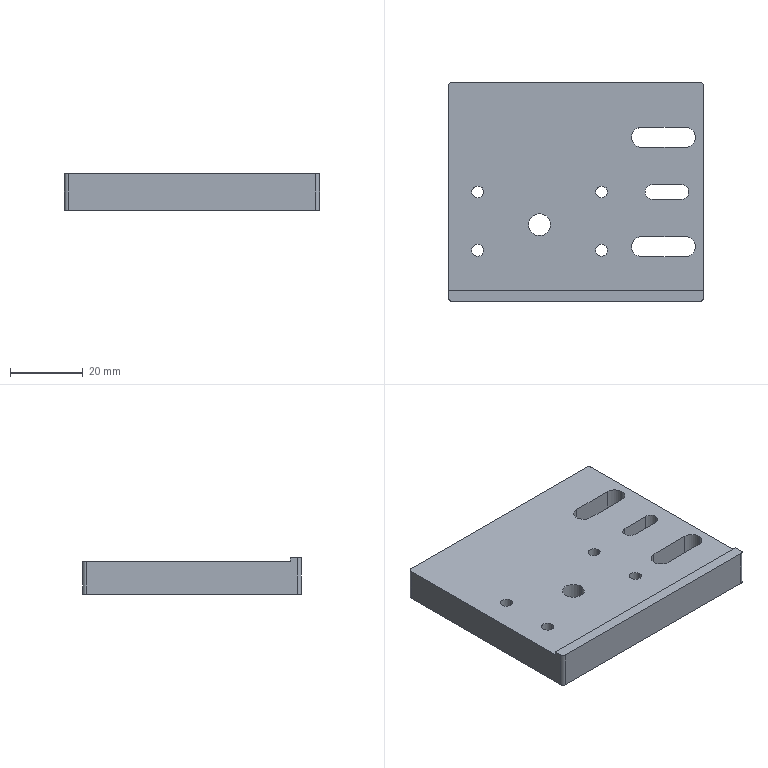Part | STEP file | 04-13 support plate A | 1 solid | 37 faces | box 70 x 60 x 10 mm | volume 35423 mm3 | cylinder 23 | plane 14 | commonest cylinder face diameters 3.3 x8 5.5 x6 2 x4 4 x3 6 x2
STEP:
#1=CARTESIAN_POINT('',(31.,0.,0.));
#2=VERTEX_POINT('',#1);
#3=CARTESIAN_POINT('',(29.,2.,0.));
#4=VERTEX_POINT('',#3);
#5=CARTESIAN_POINT('',(29.,0.,0.));
#6=DIRECTION('',(0.,0.,1.));
#7=DIRECTION('',(1.,0.,0.));
#8=AXIS2_PLACEMENT_3D('',#5,#6,#7);
#9=CIRCLE('',#8,2.);
#10=EDGE_CURVE('',#2,#4,#9,.T.);
#11=ORIENTED_EDGE('',*,*,#10,.F.);
#12=CARTESIAN_POINT('',(31.,0.,9.));
#13=VERTEX_POINT('',#12);
#14=CARTESIAN_POINT('',(31.,0.,-65.));
#15=DIRECTION('',(0.,0.,1.));
#16=VECTOR('',#15,1000.);
#17=LINE('',#14,#16);
#18=EDGE_CURVE('',#2,#13,#17,.T.);
#19=ORIENTED_EDGE('',*,*,#18,.T.);
#20=CARTESIAN_POINT('',(29.,2.,9.));
#21=VERTEX_POINT('',#20);
#22=CARTESIAN_POINT('',(29.,0.,9.));
#23=DIRECTION('',(0.,0.,1.));
#24=DIRECTION('',(1.,0.,0.));
#25=AXIS2_PLACEMENT_3D('',#22,#23,#24);
#26=CIRCLE('',#25,2.);
#27=EDGE_CURVE('',#13,#21,#26,.T.);
#28=ORIENTED_EDGE('',*,*,#27,.T.);
#29=CARTESIAN_POINT('',(29.,2.,-65.));
#30=DIRECTION('',(0.,0.,1.));
#31=VECTOR('',#30,1000.);
#32=LINE('',#29,#31);
#33=EDGE_CURVE('',#4,#21,#32,.T.);
#34=ORIENTED_EDGE('',*,*,#33,.F.);
#35=EDGE_LOOP('',(#11,#19,#28,#34));
#36=FACE_OUTER_BOUND('',#35,.T.);
#37=CARTESIAN_POINT('',(29.,0.,-65.));
#38=DIRECTION('',(0.,0.,1.));
#39=DIRECTION('',(1.,0.,0.));
#40=AXIS2_PLACEMENT_3D('',#37,#38,#39);
#41=CYLINDRICAL_SURFACE('',#40,2.);
#42=ADVANCED_FACE('',(#36),#41,.F.);
#43=CARTESIAN_POINT('',(32.75,15.,0.));
#44=VERTEX_POINT('',#43);
#45=CARTESIAN_POINT('',(30.,17.75,0.));
#46=VERTEX_POINT('',#45);
#47=CARTESIAN_POINT('',(30.,15.,0.));
#48=DIRECTION('',(0.,0.,1.));
#49=DIRECTION('',(1.,0.,0.));
#50=AXIS2_PLACEMENT_3D('',#47,#48,#49);
#51=CIRCLE('',#50,2.75);
#52=EDGE_CURVE('',#44,#46,#51,.T.);
#53=ORIENTED_EDGE('',*,*,#52,.F.);
#54=CARTESIAN_POINT('',(32.75,15.,9.));
#55=VERTEX_POINT('',#54);
#56=CARTESIAN_POINT('',(32.75,15.,-65.));
#57=DIRECTION('',(0.,0.,1.));
#58=VECTOR('',#57,1000.);
#59=LINE('',#56,#58);
#60=EDGE_CURVE('',#44,#55,#59,.T.);
#61=ORIENTED_EDGE('',*,*,#60,.T.);
#62=CARTESIAN_POINT('',(30.,17.75,9.));
#63=VERTEX_POINT('',#62);
#64=CARTESIAN_POINT('',(30.,15.,9.));
#65=DIRECTION('',(0.,0.,1.));
#66=DIRECTION('',(-1.,0.,0.));
#67=AXIS2_PLACEMENT_3D('',#64,#65,#66);
#68=CIRCLE('',#67,2.75);
#69=EDGE_CURVE('',#55,#63,#68,.T.);
#70=ORIENTED_EDGE('',*,*,#69,.T.);
#71=CARTESIAN_POINT('',(30.,17.75,-65.));
#72=DIRECTION('',(0.,0.,1.));
#73=VECTOR('',#72,1000.);
#74=LINE('',#71,#73);
#75=EDGE_CURVE('',#46,#63,#74,.T.);
#76=ORIENTED_EDGE('',*,*,#75,.F.);
#77=EDGE_LOOP('',(#53,#61,#70,#76));
#78=FACE_OUTER_BOUND('',#77,.T.);
#79=CARTESIAN_POINT('',(30.,15.,-65.));
#80=DIRECTION('',(0.,0.,1.));
#81=DIRECTION('',(1.,0.,0.));
#82=AXIS2_PLACEMENT_3D('',#79,#80,#81);
#83=CYLINDRICAL_SURFACE('',#82,2.75);
#84=ADVANCED_FACE('',(#78),#83,.F.);
#85=CARTESIAN_POINT('',(32.75,-15.,0.));
#86=VERTEX_POINT('',#85);
#87=CARTESIAN_POINT('',(30.,-12.25,0.));
#88=VERTEX_POINT('',#87);
#89=CARTESIAN_POINT('',(30.,-15.,0.));
#90=DIRECTION('',(0.,0.,1.));
#91=DIRECTION('',(1.,0.,0.));
#92=AXIS2_PLACEMENT_3D('',#89,#90,#91);
#93=CIRCLE('',#92,2.75);
#94=EDGE_CURVE('',#86,#88,#93,.T.);
#95=ORIENTED_EDGE('',*,*,#94,.F.);
#96=CARTESIAN_POINT('',(32.75,-15.,9.));
#97=VERTEX_POINT('',#96);
#98=CARTESIAN_POINT('',(32.75,-15.,-65.));
#99=DIRECTION('',(0.,0.,1.));
#100=VECTOR('',#99,1000.);
#101=LINE('',#98,#100);
#102=EDGE_CURVE('',#86,#97,#101,.T.);
#103=ORIENTED_EDGE('',*,*,#102,.T.);
#104=CARTESIAN_POINT('',(30.,-12.25,9.));
#105=VERTEX_POINT('',#104);
#106=CARTESIAN_POINT('',(30.,-15.,9.));
#107=DIRECTION('',(0.,0.,1.));
#108=DIRECTION('',(1.,0.,0.));
#109=AXIS2_PLACEMENT_3D('',#106,#107,#108);
#110=CIRCLE('',#109,2.75);
#111=EDGE_CURVE('',#97,#105,#110,.T.);
#112=ORIENTED_EDGE('',*,*,#111,.T.);
#113=CARTESIAN_POINT('',(30.,-12.25,-65.));
#114=DIRECTION('',(0.,0.,1.));
#115=VECTOR('',#114,1000.);
#116=LINE('',#113,#115);
#117=EDGE_CURVE('',#88,#105,#116,.T.);
#118=ORIENTED_EDGE('',*,*,#117,.F.);
#119=EDGE_LOOP('',(#95,#103,#112,#118));
#120=FACE_OUTER_BOUND('',#119,.T.);
#121=CARTESIAN_POINT('',(30.,-15.,-65.));
#122=DIRECTION('',(0.,0.,1.));
#123=DIRECTION('',(1.,0.,0.));
#124=AXIS2_PLACEMENT_3D('',#121,#122,#123);
#125=CYLINDRICAL_SURFACE('',#124,2.75);
#126=ADVANCED_FACE('',(#120),#125,.F.);
#127=CARTESIAN_POINT('',(-28.65,0.,0.));
#128=VERTEX_POINT('',#127);
#129=CARTESIAN_POINT('',(-25.35,0.,0.));
#130=VERTEX_POINT('',#129);
#131=CARTESIAN_POINT('',(-27.,0.,0.));
#132=DIRECTION('',(0.,0.,1.));
#133=DIRECTION('',(1.,0.,0.));
#134=AXIS2_PLACEMENT_3D('',#131,#132,#133);
#135=CIRCLE('',#134,1.65);
#136=EDGE_CURVE('',#128,#130,#135,.T.);
#137=ORIENTED_EDGE('',*,*,#136,.F.);
#138=CARTESIAN_POINT('',(-28.65,0.,9.));
#139=VERTEX_POINT('',#138);
#140=CARTESIAN_POINT('',(-28.65,0.,9.));
#141=DIRECTION('',(0.,0.,1.));
#142=VECTOR('',#141,1000.);
#143=LINE('',#140,#142);
#144=EDGE_CURVE('',#128,#139,#143,.T.);
#145=ORIENTED_EDGE('',*,*,#144,.T.);
#146=CARTESIAN_POINT('',(-25.35,0.,9.));
#147=VERTEX_POINT('',#146);
#148=CARTESIAN_POINT('',(-27.,0.,9.));
#149=DIRECTION('',(0.,0.,1.));
#150=DIRECTION('',(1.,0.,0.));
#151=AXIS2_PLACEMENT_3D('',#148,#149,#150);
#152=CIRCLE('',#151,1.65);
#153=EDGE_CURVE('',#139,#147,#152,.T.);
#154=ORIENTED_EDGE('',*,*,#153,.T.);
#155=CARTESIAN_POINT('',(-25.35,0.,9.));
#156=DIRECTION('',(0.,0.,1.));
#157=VECTOR('',#156,1000.);
#158=LINE('',#155,#157);
#159=EDGE_CURVE('',#130,#147,#158,.T.);
#160=ORIENTED_EDGE('',*,*,#159,.F.);
#161=EDGE_LOOP('',(#137,#145,#154,#160));
#162=FACE_OUTER_BOUND('',#161,.T.);
#163=CARTESIAN_POINT('',(-27.,0.,9.));
#164=DIRECTION('',(0.,0.,1.));
#165=DIRECTION('',(1.,0.,0.));
#166=AXIS2_PLACEMENT_3D('',#163,#164,#165);
#167=CYLINDRICAL_SURFACE('',#166,1.65);
#168=ADVANCED_FACE('',(#162),#167,.F.);
#169=CARTESIAN_POINT('',(-28.65,-16.,0.));
#170=VERTEX_POINT('',#169);
#171=CARTESIAN_POINT('',(-25.35,-16.,0.));
#172=VERTEX_POINT('',#171);
#173=CARTESIAN_POINT('',(-27.,-16.,0.));
#174=DIRECTION('',(0.,0.,1.));
#175=DIRECTION('',(1.,0.,0.));
#176=AXIS2_PLACEMENT_3D('',#173,#174,#175);
#177=CIRCLE('',#176,1.65);
#178=EDGE_CURVE('',#170,#172,#177,.T.);
#179=ORIENTED_EDGE('',*,*,#178,.F.);
#180=CARTESIAN_POINT('',(-28.65,-16.,9.));
#181=VERTEX_POINT('',#180);
#182=CARTESIAN_POINT('',(-28.65,-16.,9.));
#183=DIRECTION('',(0.,0.,1.));
#184=VECTOR('',#183,1000.);
#185=LINE('',#182,#184);
#186=EDGE_CURVE('',#170,#181,#185,.T.);
#187=ORIENTED_EDGE('',*,*,#186,.T.);
#188=CARTESIAN_POINT('',(-25.35,-16.,9.));
#189=VERTEX_POINT('',#188);
#190=CARTESIAN_POINT('',(-27.,-16.,9.));
#191=DIRECTION('',(0.,0.,1.));
#192=DIRECTION('',(1.,0.,0.));
#193=AXIS2_PLACEMENT_3D('',#190,#191,#192);
#194=CIRCLE('',#193,1.65);
#195=EDGE_CURVE('',#181,#189,#194,.T.);
#196=ORIENTED_EDGE('',*,*,#195,.T.);
#197=CARTESIAN_POINT('',(-25.35,-16.,9.));
#198=DIRECTION('',(0.,0.,1.));
#199=VECTOR('',#198,1000.);
#200=LINE('',#197,#199);
#201=EDGE_CURVE('',#172,#189,#200,.T.);
#202=ORIENTED_EDGE('',*,*,#201,.F.);
#203=EDGE_LOOP('',(#179,#187,#196,#202));
#204=FACE_OUTER_BOUND('',#203,.T.);
#205=CARTESIAN_POINT('',(-27.,-16.,9.));
#206=DIRECTION('',(0.,0.,1.));
#207=DIRECTION('',(1.,0.,0.));
#208=AXIS2_PLACEMENT_3D('',#205,#206,#207);
#209=CYLINDRICAL_SURFACE('',#208,1.65);
#210=ADVANCED_FACE('',(#204),#209,.F.);
#211=CARTESIAN_POINT('',(5.35,0.,0.));
#212=VERTEX_POINT('',#211);
#213=CARTESIAN_POINT('',(8.65,0.,0.));
#214=VERTEX_POINT('',#213);
#215=CARTESIAN_POINT('',(7.,0.,0.));
#216=DIRECTION('',(0.,0.,1.));
#217=DIRECTION('',(1.,0.,0.));
#218=AXIS2_PLACEMENT_3D('',#215,#216,#217);
#219=CIRCLE('',#218,1.65);
#220=EDGE_CURVE('',#212,#214,#219,.T.);
#221=ORIENTED_EDGE('',*,*,#220,.F.);
#222=CARTESIAN_POINT('',(5.35,0.,9.));
#223=VERTEX_POINT('',#222);
#224=CARTESIAN_POINT('',(5.35,0.,9.));
#225=DIRECTION('',(0.,0.,1.));
#226=VECTOR('',#225,1000.);
#227=LINE('',#224,#226);
#228=EDGE_CURVE('',#212,#223,#227,.T.);
#229=ORIENTED_EDGE('',*,*,#228,.T.);
#230=CARTESIAN_POINT('',(8.65,0.,9.));
#231=VERTEX_POINT('',#230);
#232=CARTESIAN_POINT('',(7.,0.,9.));
#233=DIRECTION('',(0.,0.,1.));
#234=DIRECTION('',(1.,0.,0.));
#235=AXIS2_PLACEMENT_3D('',#232,#233,#234);
#236=CIRCLE('',#235,1.65);
#237=EDGE_CURVE('',#223,#231,#236,.T.);
#238=ORIENTED_EDGE('',*,*,#237,.T.);
#239=CARTESIAN_POINT('',(8.65,0.,9.));
#240=DIRECTION('',(0.,0.,1.));
#241=VECTOR('',#240,1000.);
#242=LINE('',#239,#241);
#243=EDGE_CURVE('',#214,#231,#242,.T.);
#244=ORIENTED_EDGE('',*,*,#243,.F.);
#245=EDGE_LOOP('',(#221,#229,#238,#244));
#246=FACE_OUTER_BOUND('',#245,.T.);
#247=CARTESIAN_POINT('',(7.,0.,9.));
#248=DIRECTION('',(0.,0.,1.));
#249=DIRECTION('',(1.,0.,0.));
#250=AXIS2_PLACEMENT_3D('',#247,#248,#249);
#251=CYLINDRICAL_SURFACE('',#250,1.65);
#252=ADVANCED_FACE('',(#246),#251,.F.);
#253=CARTESIAN_POINT('',(5.35,-16.,0.));
#254=VERTEX_POINT('',#253);
#255=CARTESIAN_POINT('',(8.65,-16.,0.));
#256=VERTEX_POINT('',#255);
#257=CARTESIAN_POINT('',(7.,-16.,0.));
#258=DIRECTION('',(0.,0.,1.));
#259=DIRECTION('',(1.,0.,0.));
#260=AXIS2_PLACEMENT_3D('',#257,#258,#259);
#261=CIRCLE('',#260,1.65);
#262=EDGE_CURVE('',#254,#256,#261,.T.);
#263=ORIENTED_EDGE('',*,*,#262,.F.);
#264=CARTESIAN_POINT('',(5.35,-16.,9.));
#265=VERTEX_POINT('',#264);
#266=CARTESIAN_POINT('',(5.35,-16.,9.));
#267=DIRECTION('',(0.,0.,1.));
#268=VECTOR('',#267,1000.);
#269=LINE('',#266,#268);
#270=EDGE_CURVE('',#254,#265,#269,.T.);
#271=ORIENTED_EDGE('',*,*,#270,.T.);
#272=CARTESIAN_POINT('',(8.65,-16.,9.));
#273=VERTEX_POINT('',#272);
#274=CARTESIAN_POINT('',(7.,-16.,9.));
#275=DIRECTION('',(0.,0.,1.));
#276=DIRECTION('',(1.,0.,0.));
#277=AXIS2_PLACEMENT_3D('',#274,#275,#276);
#278=CIRCLE('',#277,1.65);
#279=EDGE_CURVE('',#265,#273,#278,.T.);
#280=ORIENTED_EDGE('',*,*,#279,.T.);
#281=CARTESIAN_POINT('',(8.65,-16.,9.));
#282=DIRECTION('',(0.,0.,1.));
#283=VECTOR('',#282,1000.);
#284=LINE('',#281,#283);
#285=EDGE_CURVE('',#256,#273,#284,.T.);
#286=ORIENTED_EDGE('',*,*,#285,.F.);
#287=EDGE_LOOP('',(#263,#271,#280,#286));
#288=FACE_OUTER_BOUND('',#287,.T.);
#289=CARTESIAN_POINT('',(7.,-16.,9.));
#290=DIRECTION('',(0.,0.,1.));
#291=DIRECTION('',(1.,0.,0.));
#292=AXIS2_PLACEMENT_3D('',#289,#290,#291);
#293=CYLINDRICAL_SURFACE('',#292,1.65);
#294=ADVANCED_FACE('',(#288),#293,.F.);
#295=CARTESIAN_POINT('',(-13.,-9.,0.));
#296=VERTEX_POINT('',#295);
#297=CARTESIAN_POINT('',(-7.,-9.,0.));
#298=VERTEX_POINT('',#297);
#299=CARTESIAN_POINT('',(-10.,-9.,0.));
#300=DIRECTION('',(0.,0.,1.));
#301=DIRECTION('',(1.,0.,0.));
#302=AXIS2_PLACEMENT_3D('',#299,#300,#301);
#303=CIRCLE('',#302,3.);
#304=EDGE_CURVE('',#296,#298,#303,.T.);
#305=ORIENTED_EDGE('',*,*,#304,.F.);
#306=CARTESIAN_POINT('',(-13.,-9.,9.));
#307=VERTEX_POINT('',#306);
#308=CARTESIAN_POINT('',(-13.,-9.,-65.));
#309=DIRECTION('',(0.,0.,1.));
#310=VECTOR('',#309,1000.);
#311=LINE('',#308,#310);
#312=EDGE_CURVE('',#296,#307,#311,.T.);
#313=ORIENTED_EDGE('',*,*,#312,.T.);
#314=CARTESIAN_POINT('',(-7.,-9.,9.));
#315=VERTEX_POINT('',#314);
#316=CARTESIAN_POINT('',(-10.,-9.,9.));
#317=DIRECTION('',(0.,0.,1.));
#318=DIRECTION('',(1.,0.,0.));
#319=AXIS2_PLACEMENT_3D('',#316,#317,#318);
#320=CIRCLE('',#319,3.);
#321=EDGE_CURVE('',#307,#315,#320,.T.);
#322=ORIENTED_EDGE('',*,*,#321,.T.);
#323=CARTESIAN_POINT('',(-7.,-9.,-65.));
#324=DIRECTION('',(0.,0.,1.));
#325=VECTOR('',#324,1000.);
#326=LINE('',#323,#325);
#327=EDGE_CURVE('',#298,#315,#326,.T.);
#328=ORIENTED_EDGE('',*,*,#327,.F.);
#329=EDGE_LOOP('',(#305,#313,#322,#328));
#330=FACE_OUTER_BOUND('',#329,.T.);
#331=CARTESIAN_POINT('',(-10.,-9.,-65.));
#332=DIRECTION('',(0.,0.,1.));
#333=DIRECTION('',(1.,0.,0.));
#334=AXIS2_PLACEMENT_3D('',#331,#332,#333);
#335=CYLINDRICAL_SURFACE('',#334,3.);
#336=ADVANCED_FACE('',(#330),#335,.F.);
#337=CARTESIAN_POINT('',(35.,-29.,0.));
#338=VERTEX_POINT('',#337);
#339=CARTESIAN_POINT('',(35.,29.,0.));
#340=VERTEX_POINT('',#339);
#341=CARTESIAN_POINT('',(35.,30.,0.));
#342=DIRECTION('',(0.,1.,0.));
#343=VECTOR('',#342,1000.);
#344=LINE('',#341,#343);
#345=EDGE_CURVE('',#338,#340,#344,.T.);
#346=ORIENTED_EDGE('',*,*,#345,.T.);
#347=CARTESIAN_POINT('',(35.,29.,9.));
#348=VERTEX_POINT('',#347);
#349=CARTESIAN_POINT('',(35.,29.,10.));
#350=DIRECTION('',(0.,0.,1.));
#351=VECTOR('',#350,1000.);
#352=LINE('',#349,#351);
#353=EDGE_CURVE('',#340,#348,#352,.T.);
#354=ORIENTED_EDGE('',*,*,#353,.T.);
#355=CARTESIAN_POINT('',(35.,-27.,9.));
#356=VERTEX_POINT('',#355);
#357=CARTESIAN_POINT('',(35.,30.,9.));
#358=DIRECTION('',(0.,-1.,0.));
#359=VECTOR('',#358,1000.);
#360=LINE('',#357,#359);
#361=EDGE_CURVE('',#348,#356,#360,.T.);
#362=ORIENTED_EDGE('',*,*,#361,.T.);
#363=CARTESIAN_POINT('',(35.,-27.,10.));
#364=VERTEX_POINT('',#363);
#365=CARTESIAN_POINT('',(35.,-27.,10.));
#366=DIRECTION('',(0.,0.,1.));
#367=VECTOR('',#366,1000.);
#368=LINE('',#365,#367);
#369=EDGE_CURVE('',#356,#364,#368,.T.);
#370=ORIENTED_EDGE('',*,*,#369,.T.);
#371=CARTESIAN_POINT('',(35.,-29.,10.));
#372=VERTEX_POINT('',#371);
#373=CARTESIAN_POINT('',(35.,30.,10.));
#374=DIRECTION('',(0.,1.,0.));
#375=VECTOR('',#374,1000.);
#376=LINE('',#373,#375);
#377=EDGE_CURVE('',#372,#364,#376,.T.);
#378=ORIENTED_EDGE('',*,*,#377,.F.);
#379=CARTESIAN_POINT('',(35.,-29.,10.));
#380=DIRECTION('',(0.,0.,-1.));
#381=VECTOR('',#380,1000.);
#382=LINE('',#379,#381);
#383=EDGE_CURVE('',#372,#338,#382,.T.);
#384=ORIENTED_EDGE('',*,*,#383,.T.);
#385=EDGE_LOOP('',(#346,#354,#362,#370,#378,#384));
#386=FACE_OUTER_BOUND('',#385,.T.);
#387=CARTESIAN_POINT('',(35.,30.,10.));
#388=DIRECTION('',(-1.,0.,0.));
#389=DIRECTION('',(0.,-1.,0.));
#390=AXIS2_PLACEMENT_3D('',#387,#388,#389);
#391=PLANE('',#390);
#392=ADVANCED_FACE('',(#386),#391,.F.);
#393=CARTESIAN_POINT('',(-34.,30.,9.));
#394=VERTEX_POINT('',#393);
#395=CARTESIAN_POINT('',(34.,30.,9.));
#396=VERTEX_POINT('',#395);
#397=CARTESIAN_POINT('',(-35.,30.,9.));
#398=DIRECTION('',(1.,0.,0.));
#399=VECTOR('',#398,1000.);
#400=LINE('',#397,#399);
#401=EDGE_CURVE('',#394,#396,#400,.T.);
#402=ORIENTED_EDGE('',*,*,#401,.T.);
#403=CARTESIAN_POINT('',(34.,30.,0.));
#404=VERTEX_POINT('',#403);
#405=CARTESIAN_POINT('',(34.,30.,10.));
#406=DIRECTION('',(0.,0.,-1.));
#407=VECTOR('',#406,1000.);
#408=LINE('',#405,#407);
#409=EDGE_CURVE('',#396,#404,#408,.T.);
#410=ORIENTED_EDGE('',*,*,#409,.T.);
#411=CARTESIAN_POINT('',(-34.,30.,0.));
#412=VERTEX_POINT('',#411);
#413=CARTESIAN_POINT('',(-35.,30.,0.));
#414=DIRECTION('',(-1.,0.,0.));
#415=VECTOR('',#414,1000.);
#416=LINE('',#413,#415);
#417=EDGE_CURVE('',#404,#412,#416,.T.);
#418=ORIENTED_EDGE('',*,*,#417,.T.);
#419=CARTESIAN_POINT('',(-34.,30.,10.));
#420=DIRECTION('',(0.,0.,1.));
#421=VECTOR('',#420,1000.);
#422=LINE('',#419,#421);
#423=EDGE_CURVE('',#412,#394,#422,.T.);
#424=ORIENTED_EDGE('',*,*,#423,.T.);
#425=EDGE_LOOP('',(#402,#410,#418,#424));
#426=FACE_OUTER_BOUND('',#425,.T.);
#427=CARTESIAN_POINT('',(-35.,30.,10.));
#428=DIRECTION('',(0.,-1.,0.));
#429=DIRECTION('',(0.,0.,-1.));
#430=AXIS2_PLACEMENT_3D('',#427,#428,#429);
#431=PLANE('',#430);
#432=ADVANCED_FACE('',(#426),#431,.F.);
#433=CARTESIAN_POINT('',(-35.,29.,9.));
#434=VERTEX_POINT('',#433);
#435=CARTESIAN_POINT('',(-35.,-27.,9.));
#436=VERTEX_POINT('',#435);
#437=CARTESIAN_POINT('',(-35.,-27.,9.));
#438=DIRECTION('',(0.,-1.,0.));
#439=VECTOR('',#438,1000.);
#440=LINE('',#437,#439);
#441=EDGE_CURVE('',#434,#436,#440,.T.);
#442=ORIENTED_EDGE('',*,*,#441,.F.);
#443=CARTESIAN_POINT('',(-35.,29.,0.));
#444=VERTEX_POINT('',#443);
#445=CARTESIAN_POINT('',(-35.,29.,10.));
#446=DIRECTION('',(0.,0.,-1.));
#447=VECTOR('',#446,1000.);
#448=LINE('',#445,#447);
#449=EDGE_CURVE('',#434,#444,#448,.T.);
#450=ORIENTED_EDGE('',*,*,#449,.T.);
#451=CARTESIAN_POINT('',(-35.,-29.,0.));
#452=VERTEX_POINT('',#451);
#453=CARTESIAN_POINT('',(-35.,30.,0.));
#454=DIRECTION('',(0.,-1.,0.));
#455=VECTOR('',#454,1000.);
#456=LINE('',#453,#455);
#457=EDGE_CURVE('',#444,#452,#456,.T.);
#458=ORIENTED_EDGE('',*,*,#457,.T.);
#459=CARTESIAN_POINT('',(-35.,-29.,10.));
#460=VERTEX_POINT('',#459);
#461=CARTESIAN_POINT('',(-35.,-29.,10.));
#462=DIRECTION('',(0.,0.,1.));
#463=VECTOR('',#462,1000.);
#464=LINE('',#461,#463);
#465=EDGE_CURVE('',#452,#460,#464,.T.);
#466=ORIENTED_EDGE('',*,*,#465,.T.);
#467=CARTESIAN_POINT('',(-35.,-27.,10.));
#468=VERTEX_POINT('',#467);
#469=CARTESIAN_POINT('',(-35.,30.,10.));
#470=DIRECTION('',(0.,-1.,0.));
#471=VECTOR('',#470,1000.);
#472=LINE('',#469,#471);
#473=EDGE_CURVE('',#468,#460,#472,.T.);
#474=ORIENTED_EDGE('',*,*,#473,.F.);
#475=CARTESIAN_POINT('',(-35.,-27.,9.));
#476=DIRECTION('',(0.,0.,1.));
#477=VECTOR('',#476,1000.);
#478=LINE('',#475,#477);
#479=EDGE_CURVE('',#436,#468,#478,.T.);
#480=ORIENTED_EDGE('',*,*,#479,.F.);
#481=EDGE_LOOP('',(#442,#450,#458,#466,#474,#480));
#482=FACE_OUTER_BOUND('',#481,.T.);
#483=CARTESIAN_POINT('',(-35.,30.,10.));
#484=DIRECTION('',(1.,0.,0.));
#485=DIRECTION('',(0.,1.,0.));
#486=AXIS2_PLACEMENT_3D('',#483,#484,#485);
#487=PLANE('',#486);
#488=ADVANCED_FACE('',(#482),#487,.F.);
#489=CARTESIAN_POINT('',(-34.,-30.,0.));
#490=VERTEX_POINT('',#489);
#491=CARTESIAN_POINT('',(34.,-30.,0.));
#492=VERTEX_POINT('',#491);
#493=CARTESIAN_POINT('',(-35.,-30.,0.));
#494=DIRECTION('',(1.,0.,0.));
#495=VECTOR('',#494,1000.);
#496=LINE('',#493,#495);
#497=EDGE_CURVE('',#490,#492,#496,.T.);
#498=ORIENTED_EDGE('',*,*,#497,.T.);
#499=CARTESIAN_POINT('',(34.,-30.,10.));
#500=VERTEX_POINT('',#499);
#501=CARTESIAN_POINT('',(34.,-30.,10.));
#502=DIRECTION('',(0.,0.,1.));
#503=VECTOR('',#502,1000.);
#504=LINE('',#501,#503);
#505=EDGE_CURVE('',#492,#500,#504,.T.);
#506=ORIENTED_EDGE('',*,*,#505,.T.);
#507=CARTESIAN_POINT('',(-34.,-30.,10.));
#508=VERTEX_POINT('',#507);
#509=CARTESIAN_POINT('',(-35.,-30.,10.));
#510=DIRECTION('',(1.,0.,0.));
#511=VECTOR('',#510,1000.);
#512=LINE('',#509,#511);
#513=EDGE_CURVE('',#508,#500,#512,.T.);
#514=ORIENTED_EDGE('',*,*,#513,.F.);
#515=CARTESIAN_POINT('',(-34.,-30.,10.));
#516=DIRECTION('',(0.,0.,-1.));
#517=VECTOR('',#516,1000.);
#518=LINE('',#515,#517);
#519=EDGE_CURVE('',#508,#490,#518,.T.);
#520=ORIENTED_EDGE('',*,*,#519,.T.);
#521=EDGE_LOOP('',(#498,#506,#514,#520));
#522=FACE_OUTER_BOUND('',#521,.T.);
#523=CARTESIAN_POINT('',(-35.,-30.,10.));
#524=DIRECTION('',(0.,1.,0.));
#525=DIRECTION('',(0.,0.,1.));
#526=AXIS2_PLACEMENT_3D('',#523,#524,#525);
#527=PLANE('',#526);
#528=ADVANCED_FACE('',(#522),#527,.F.);
#529=ORIENTED_EDGE('',*,*,#513,.T.);
#530=CARTESIAN_POINT('',(34.,-29.,10.));
#531=DIRECTION('',(0.,0.,1.));
#532=DIRECTION('',(1.,0.,0.));
#533=AXIS2_PLACEMENT_3D('',#530,#531,#532);
#534=CIRCLE('',#533,1.);
#535=EDGE_CURVE('',#500,#372,#534,.T.);
#536=ORIENTED_EDGE('',*,*,#535,.T.);
#537=ORIENTED_EDGE('',*,*,#377,.T.);
#538=CARTESIAN_POINT('',(35.,-27.,10.));
#539=DIRECTION('',(1.,0.,0.));
#540=VECTOR('',#539,1000.);
#541=LINE('',#538,#540);
#542=EDGE_CURVE('',#468,#364,#541,.T.);
#543=ORIENTED_EDGE('',*,*,#542,.F.);
#544=ORIENTED_EDGE('',*,*,#473,.T.);
#545=CARTESIAN_POINT('',(-34.,-29.,10.));
#546=DIRECTION('',(0.,0.,1.));
#547=DIRECTION('',(1.,0.,0.));
#548=AXIS2_PLACEMENT_3D('',#545,#546,#547);
#549=CIRCLE('',#548,1.);
#550=EDGE_CURVE('',#460,#508,#549,.T.);
#551=ORIENTED_EDGE('',*,*,#550,.T.);
#552=EDGE_LOOP('',(#529,#536,#537,#543,#544,#551));
#553=FACE_OUTER_BOUND('',#552,.T.);
#554=CARTESIAN_POINT('',(35.,-30.,10.));
#555=DIRECTION('',(0.,0.,1.));
#556=DIRECTION('',(1.,0.,0.));
#557=AXIS2_PLACEMENT_3D('',#554,#555,#556);
#558=PLANE('',#557);
#559=ADVANCED_FACE('',(#553),#558,.T.);
#560=CARTESIAN_POINT('',(21.,2.,0.));
#561=VERTEX_POINT('',#560);
#562=CARTESIAN_POINT('',(35.,2.,0.));
#563=DIRECTION('',(-1.,0.,0.));
#564=VECTOR('',#563,1000.);
#565=LINE('',#562,#564);
#566=EDGE_CURVE('',#4,#561,#565,.T.);
#567=ORIENTED_EDGE('',*,*,#566,.T.);
#568=CARTESIAN_POINT('',(21.,-2.,0.));
#569=VERTEX_POINT('',#568);
#570=CARTESIAN_POINT('',(21.,0.,0.));
#571=DIRECTION('',(0.,0.,1.));
#572=DIRECTION('',(1.,0.,0.));
#573=AXIS2_PLACEMENT_3D('',#570,#571,#572);
#574=CIRCLE('',#573,2.);
#575=EDGE_CURVE('',#561,#569,#574,.T.);
#576=ORIENTED_EDGE('',*,*,#575,.T.);
#577=CARTESIAN_POINT('',(29.,-2.,0.));
#578=VERTEX_POINT('',#577);
#579=CARTESIAN_POINT('',(35.,-2.,0.));
#580=DIRECTION('',(1.,0.,0.));
#581=VECTOR('',#580,1000.);
#582=LINE('',#579,#581);
#583=EDGE_CURVE('',#569,#578,#582,.T.);
#584=ORIENTED_EDGE('',*,*,#583,.T.);
#585=CARTESIAN_POINT('',(29.,0.,0.));
#586=DIRECTION('',(0.,0.,1.));
#587=DIRECTION('',(1.,0.,0.));
#588=AXIS2_PLACEMENT_3D('',#585,#586,#587);
#589=CIRCLE('',#588,2.);
#590=EDGE_CURVE('',#578,#2,#589,.T.);
#591=ORIENTED_EDGE('',*,*,#590,.T.);
#592=ORIENTED_EDGE('',*,*,#10,.T.);
#593=EDGE_LOOP('',(#567,#576,#584,#591,#592));
#594=FACE_BOUND('',#593,.T.);
#595=CARTESIAN_POINT('',(18.,17.75,0.));
#596=VERTEX_POINT('',#595);
#597=CARTESIAN_POINT('',(35.,17.75,0.));
#598=DIRECTION('',(-1.,0.,0.));
#599=VECTOR('',#598,1000.);
#600=LINE('',#597,#599);
#601=EDGE_CURVE('',#46,#596,#600,.T.);
#602=ORIENTED_EDGE('',*,*,#601,.T.);
#603=CARTESIAN_POINT('',(18.,12.25,0.));
#604=VERTEX_POINT('',#603);
#605=CARTESIAN_POINT('',(18.,15.,0.));
#606=DIRECTION('',(0.,0.,1.));
#607=DIRECTION('',(1.,0.,0.));
#608=AXIS2_PLACEMENT_3D('',#605,#606,#607);
#609=CIRCLE('',#608,2.75);
#610=EDGE_CURVE('',#596,#604,#609,.T.);
#611=ORIENTED_EDGE('',*,*,#610,.T.);
#612=CARTESIAN_POINT('',(30.,12.25,0.));
#613=VERTEX_POINT('',#612);
#614=CARTESIAN_POINT('',(35.,12.25,0.));
#615=DIRECTION('',(1.,0.,0.));
#616=VECTOR('',#615,1000.);
#617=LINE('',#614,#616);
#618=EDGE_CURVE('',#604,#613,#617,.T.);
#619=ORIENTED_EDGE('',*,*,#618,.T.);
#620=CARTESIAN_POINT('',(30.,15.,0.));
#621=DIRECTION('',(0.,0.,1.));
#622=DIRECTION('',(1.,0.,0.));
#623=AXIS2_PLACEMENT_3D('',#620,#621,#622);
#624=CIRCLE('',#623,2.75);
#625=EDGE_CURVE('',#613,#44,#624,.T.);
#626=ORIENTED_EDGE('',*,*,#625,.T.);
#627=ORIENTED_EDGE('',*,*,#52,.T.);
#628=EDGE_LOOP('',(#602,#611,#619,#626,#627));
#629=FACE_BOUND('',#628,.T.);
#630=CARTESIAN_POINT('',(18.,-12.25,0.));
#631=VERTEX_POINT('',#630);
#632=CARTESIAN_POINT('',(35.,-12.25,0.));
#633=DIRECTION('',(-1.,0.,0.));
#634=VECTOR('',#633,1000.);
#635=LINE('',#632,#634);
#636=EDGE_CURVE('',#88,#631,#635,.T.);
#637=ORIENTED_EDGE('',*,*,#636,.T.);
#638=CARTESIAN_POINT('',(18.,-17.75,0.));
#639=VERTEX_POINT('',#638);
#640=CARTESIAN_POINT('',(18.,-15.,0.));
#641=DIRECTION('',(0.,0.,1.));
#642=DIRECTION('',(1.,0.,0.));
#643=AXIS2_PLACEMENT_3D('',#640,#641,#642);
#644=CIRCLE('',#643,2.75);
#645=EDGE_CURVE('',#631,#639,#644,.T.);
#646=ORIENTED_EDGE('',*,*,#645,.T.);
#647=CARTESIAN_POINT('',(30.,-17.75,0.));
#648=VERTEX_POINT('',#647);
#649=CARTESIAN_POINT('',(35.,-17.75,0.));
#650=DIRECTION('',(1.,0.,0.));
#651=VECTOR('',#650,1000.);
#652=LINE('',#649,#651);
#653=EDGE_CURVE('',#639,#648,#652,.T.);
#654=ORIENTED_EDGE('',*,*,#653,.T.);
#655=CARTESIAN_POINT('',(30.,-15.,0.));
#656=DIRECTION('',(0.,0.,1.));
#657=DIRECTION('',(1.,0.,0.));
#658=AXIS2_PLACEMENT_3D('',#655,#656,#657);
#659=CIRCLE('',#658,2.75);
#660=EDGE_CURVE('',#648,#86,#659,.T.);
#661=ORIENTED_EDGE('',*,*,#660,.T.);
#662=ORIENTED_EDGE('',*,*,#94,.T.);
#663=EDGE_LOOP('',(#637,#646,#654,#661,#662));
#664=FACE_BOUND('',#663,.T.);
#665=CARTESIAN_POINT('',(-27.,0.,0.));
#666=DIRECTION('',(0.,0.,1.));
#667=DIRECTION('',(1.,0.,0.));
#668=AXIS2_PLACEMENT_3D('',#665,#666,#667);
#669=CIRCLE('',#668,1.65);
#670=EDGE_CURVE('',#130,#128,#669,.T.);
#671=ORIENTED_EDGE('',*,*,#670,.T.);
#672=ORIENTED_EDGE('',*,*,#136,.T.);
#673=EDGE_LOOP('',(#671,#672));
#674=FACE_BOUND('',#673,.T.);
#675=CARTESIAN_POINT('',(-27.,-16.,0.));
#676=DIRECTION('',(0.,0.,1.));
#677=DIRECTION('',(1.,0.,0.));
#678=AXIS2_PLACEMENT_3D('',#675,#676,#677);
#679=CIRCLE('',#678,1.65);
#680=EDGE_CURVE('',#172,#170,#679,.T.);
#681=ORIENTED_EDGE('',*,*,#680,.T.);
#682=ORIENTED_EDGE('',*,*,#178,.T.);
#683=EDGE_LOOP('',(#681,#682));
#684=FACE_BOUND('',#683,.T.);
#685=CARTESIAN_POINT('',(7.,0.,0.));
#686=DIRECTION('',(0.,0.,1.));
#687=DIRECTION('',(1.,0.,0.));
#688=AXIS2_PLACEMENT_3D('',#685,#686,#687);
#689=CIRCLE('',#688,1.65);
#690=EDGE_CURVE('',#214,#212,#689,.T.);
#691=ORIENTED_EDGE('',*,*,#690,.T.);
#692=ORIENTED_EDGE('',*,*,#220,.T.);
#693=EDGE_LOOP('',(#691,#692));
#694=FACE_BOUND('',#693,.T.);
#695=CARTESIAN_POINT('',(7.,-16.,0.));
#696=DIRECTION('',(0.,0.,1.));
#697=DIRECTION('',(1.,0.,0.));
#698=AXIS2_PLACEMENT_3D('',#695,#696,#697);
#699=CIRCLE('',#698,1.65);
#700=EDGE_CURVE('',#256,#254,#699,.T.);
#701=ORIENTED_EDGE('',*,*,#700,.T.);
#702=ORIENTED_EDGE('',*,*,#262,.T.);
#703=EDGE_LOOP('',(#701,#702));
#704=FACE_BOUND('',#703,.T.);
#705=CARTESIAN_POINT('',(-10.,-9.,0.));
#706=DIRECTION('',(0.,0.,1.));
#707=DIRECTION('',(1.,0.,0.));
#708=AXIS2_PLACEMENT_3D('',#705,#706,#707);
#709=CIRCLE('',#708,3.);
#710=EDGE_CURVE('',#298,#296,#709,.T.);
#711=ORIENTED_EDGE('',*,*,#710,.T.);
#712=ORIENTED_EDGE('',*,*,#304,.T.);
#713=EDGE_LOOP('',(#711,#712));
#714=FACE_BOUND('',#713,.T.);
#715=ORIENTED_EDGE('',*,*,#417,.F.);
#716=CARTESIAN_POINT('',(34.,29.,0.));
#717=DIRECTION('',(0.,0.,-1.));
#718=DIRECTION('',(1.,0.,0.));
#719=AXIS2_PLACEMENT_3D('',#716,#717,#718);
#720=CIRCLE('',#719,1.);
#721=EDGE_CURVE('',#404,#340,#720,.T.);
#722=ORIENTED_EDGE('',*,*,#721,.T.);
#723=ORIENTED_EDGE('',*,*,#345,.F.);
#724=CARTESIAN_POINT('',(34.,-29.,0.));
#725=DIRECTION('',(0.,0.,-1.));
#726=DIRECTION('',(1.,0.,0.));
#727=AXIS2_PLACEMENT_3D('',#724,#725,#726);
#728=CIRCLE('',#727,1.);
#729=EDGE_CURVE('',#338,#492,#728,.T.);
#730=ORIENTED_EDGE('',*,*,#729,.T.);
#731=ORIENTED_EDGE('',*,*,#497,.F.);
#732=CARTESIAN_POINT('',(-34.,-29.,0.));
#733=DIRECTION('',(0.,0.,-1.));
#734=DIRECTION('',(1.,0.,0.));
#735=AXIS2_PLACEMENT_3D('',#732,#733,#734);
#736=CIRCLE('',#735,1.);
#737=EDGE_CURVE('',#490,#452,#736,.T.);
#738=ORIENTED_EDGE('',*,*,#737,.T.);
#739=ORIENTED_EDGE('',*,*,#457,.F.);
#740=CARTESIAN_POINT('',(-34.,29.,0.));
#741=DIRECTION('',(0.,0.,-1.));
#742=DIRECTION('',(1.,0.,0.));
#743=AXIS2_PLACEMENT_3D('',#740,#741,#742);
#744=CIRCLE('',#743,1.);
#745=EDGE_CURVE('',#444,#412,#744,.T.);
#746=ORIENTED_EDGE('',*,*,#745,.T.);
#747=EDGE_LOOP('',(#715,#722,#723,#730,#731,#738,#739,#746));
#748=FACE_OUTER_BOUND('',#747,.T.);
#749=CARTESIAN_POINT('',(35.,-30.,0.));
#750=DIRECTION('',(0.,0.,1.));
#751=DIRECTION('',(1.,0.,0.));
#752=AXIS2_PLACEMENT_3D('',#749,#750,#751);
#753=PLANE('',#752);
#754=ADVANCED_FACE('',(#594,#629,#664,#674,#684,#694,#704,#714,#748),#753,.F.);
#755=CARTESIAN_POINT('',(21.,-2.,9.));
#756=VERTEX_POINT('',#755);
#757=CARTESIAN_POINT('',(29.,-2.,9.));
#758=VERTEX_POINT('',#757);
#759=CARTESIAN_POINT('',(21.,-2.,9.));
#760=DIRECTION('',(1.,0.,0.));
#761=VECTOR('',#760,1000.);
#762=LINE('',#759,#761);
#763=EDGE_CURVE('',#756,#758,#762,.T.);
#764=ORIENTED_EDGE('',*,*,#763,.F.);
#765=CARTESIAN_POINT('',(21.,2.,9.));
#766=VERTEX_POINT('',#765);
#767=CARTESIAN_POINT('',(21.,0.,9.));
#768=DIRECTION('',(0.,0.,1.));
#769=DIRECTION('',(1.,0.,0.));
#770=AXIS2_PLACEMENT_3D('',#767,#768,#769);
#771=CIRCLE('',#770,2.);
#772=EDGE_CURVE('',#766,#756,#771,.T.);
#773=ORIENTED_EDGE('',*,*,#772,.F.);
#774=CARTESIAN_POINT('',(21.,2.,9.));
#775=DIRECTION('',(-1.,0.,0.));
#776=VECTOR('',#775,1000.);
#777=LINE('',#774,#776);
#778=EDGE_CURVE('',#21,#766,#777,.T.);
#779=ORIENTED_EDGE('',*,*,#778,.F.);
#780=ORIENTED_EDGE('',*,*,#27,.F.);
#781=CARTESIAN_POINT('',(29.,0.,9.));
#782=DIRECTION('',(0.,0.,1.));
#783=DIRECTION('',(1.,0.,0.));
#784=AXIS2_PLACEMENT_3D('',#781,#782,#783);
#785=CIRCLE('',#784,2.);
#786=EDGE_CURVE('',#758,#13,#785,.T.);
#787=ORIENTED_EDGE('',*,*,#786,.F.);
#788=EDGE_LOOP('',(#764,#773,#779,#780,#787));
#789=FACE_BOUND('',#788,.T.);
#790=CARTESIAN_POINT('',(18.,12.25,9.));
#791=VERTEX_POINT('',#790);
#792=CARTESIAN_POINT('',(30.,12.25,9.));
#793=VERTEX_POINT('',#792);
#794=CARTESIAN_POINT('',(18.,12.25,9.));
#795=DIRECTION('',(1.,0.,0.));
#796=VECTOR('',#795,1000.);
#797=LINE('',#794,#796);
#798=EDGE_CURVE('',#791,#793,#797,.T.);
#799=ORIENTED_EDGE('',*,*,#798,.F.);
#800=CARTESIAN_POINT('',(18.,17.75,9.));
#801=VERTEX_POINT('',#800);
#802=CARTESIAN_POINT('',(18.,15.,9.));
#803=DIRECTION('',(0.,0.,1.));
#804=DIRECTION('',(-1.,0.,0.));
#805=AXIS2_PLACEMENT_3D('',#802,#803,#804);
#806=CIRCLE('',#805,2.75);
#807=EDGE_CURVE('',#801,#791,#806,.T.);
#808=ORIENTED_EDGE('',*,*,#807,.F.);
#809=CARTESIAN_POINT('',(18.,17.75,9.));
#810=DIRECTION('',(-1.,0.,0.));
#811=VECTOR('',#810,1000.);
#812=LINE('',#809,#811);
#813=EDGE_CURVE('',#63,#801,#812,.T.);
#814=ORIENTED_EDGE('',*,*,#813,.F.);
#815=ORIENTED_EDGE('',*,*,#69,.F.);
#816=CARTESIAN_POINT('',(30.,15.,9.));
#817=DIRECTION('',(0.,0.,1.));
#818=DIRECTION('',(-1.,0.,0.));
#819=AXIS2_PLACEMENT_3D('',#816,#817,#818);
#820=CIRCLE('',#819,2.75);
#821=EDGE_CURVE('',#793,#55,#820,.T.);
#822=ORIENTED_EDGE('',*,*,#821,.F.);
#823=EDGE_LOOP('',(#799,#808,#814,#815,#822));
#824=FACE_BOUND('',#823,.T.);
#825=CARTESIAN_POINT('',(18.,-17.75,9.));
#826=VERTEX_POINT('',#825);
#827=CARTESIAN_POINT('',(30.,-17.75,9.));
#828=VERTEX_POINT('',#827);
#829=CARTESIAN_POINT('',(18.,-17.75,9.));
#830=DIRECTION('',(1.,0.,0.));
#831=VECTOR('',#830,1000.);
#832=LINE('',#829,#831);
#833=EDGE_CURVE('',#826,#828,#832,.T.);
#834=ORIENTED_EDGE('',*,*,#833,.F.);
#835=CARTESIAN_POINT('',(18.,-12.25,9.));
#836=VERTEX_POINT('',#835);
#837=CARTESIAN_POINT('',(18.,-15.,9.));
#838=DIRECTION('',(0.,0.,1.));
#839=DIRECTION('',(1.,0.,0.));
#840=AXIS2_PLACEMENT_3D('',#837,#838,#839);
#841=CIRCLE('',#840,2.75);
#842=EDGE_CURVE('',#836,#826,#841,.T.);
#843=ORIENTED_EDGE('',*,*,#842,.F.);
#844=CARTESIAN_POINT('',(18.,-12.25,9.));
#845=DIRECTION('',(-1.,0.,0.));
#846=VECTOR('',#845,1000.);
#847=LINE('',#844,#846);
#848=EDGE_CURVE('',#105,#836,#847,.T.);
#849=ORIENTED_EDGE('',*,*,#848,.F.);
#850=ORIENTED_EDGE('',*,*,#111,.F.);
#851=CARTESIAN_POINT('',(30.,-15.,9.));
#852=DIRECTION('',(0.,0.,1.));
#853=DIRECTION('',(1.,0.,0.));
#854=AXIS2_PLACEMENT_3D('',#851,#852,#853);
#855=CIRCLE('',#854,2.75);
#856=EDGE_CURVE('',#828,#97,#855,.T.);
#857=ORIENTED_EDGE('',*,*,#856,.F.);
#858=EDGE_LOOP('',(#834,#843,#849,#850,#857));
#859=FACE_BOUND('',#858,.T.);
#860=CARTESIAN_POINT('',(-27.,0.,9.));
#861=DIRECTION('',(0.,0.,1.));
#862=DIRECTION('',(1.,0.,0.));
#863=AXIS2_PLACEMENT_3D('',#860,#861,#862);
#864=CIRCLE('',#863,1.65);
#865=EDGE_CURVE('',#147,#139,#864,.T.);
#866=ORIENTED_EDGE('',*,*,#865,.F.);
#867=ORIENTED_EDGE('',*,*,#153,.F.);
#868=EDGE_LOOP('',(#866,#867));
#869=FACE_BOUND('',#868,.T.);
#870=CARTESIAN_POINT('',(-27.,-16.,9.));
#871=DIRECTION('',(0.,0.,1.));
#872=DIRECTION('',(1.,0.,0.));
#873=AXIS2_PLACEMENT_3D('',#870,#871,#872);
#874=CIRCLE('',#873,1.65);
#875=EDGE_CURVE('',#189,#181,#874,.T.);
#876=ORIENTED_EDGE('',*,*,#875,.F.);
#877=ORIENTED_EDGE('',*,*,#195,.F.);
#878=EDGE_LOOP('',(#876,#877));
#879=FACE_BOUND('',#878,.T.);
#880=CARTESIAN_POINT('',(7.,0.,9.));
#881=DIRECTION('',(0.,0.,1.));
#882=DIRECTION('',(1.,0.,0.));
#883=AXIS2_PLACEMENT_3D('',#880,#881,#882);
#884=CIRCLE('',#883,1.65);
#885=EDGE_CURVE('',#231,#223,#884,.T.);
#886=ORIENTED_EDGE('',*,*,#885,.F.);
#887=ORIENTED_EDGE('',*,*,#237,.F.);
#888=EDGE_LOOP('',(#886,#887));
#889=FACE_BOUND('',#888,.T.);
#890=CARTESIAN_POINT('',(7.,-16.,9.));
#891=DIRECTION('',(0.,0.,1.));
#892=DIRECTION('',(1.,0.,0.));
#893=AXIS2_PLACEMENT_3D('',#890,#891,#892);
#894=CIRCLE('',#893,1.65);
#895=EDGE_CURVE('',#273,#265,#894,.T.);
#896=ORIENTED_EDGE('',*,*,#895,.F.);
#897=ORIENTED_EDGE('',*,*,#279,.F.);
#898=EDGE_LOOP('',(#896,#897));
#899=FACE_BOUND('',#898,.T.);
#900=CARTESIAN_POINT('',(-10.,-9.,9.));
#901=DIRECTION('',(0.,0.,1.));
#902=DIRECTION('',(1.,0.,0.));
#903=AXIS2_PLACEMENT_3D('',#900,#901,#902);
#904=CIRCLE('',#903,3.);
#905=EDGE_CURVE('',#315,#307,#904,.T.);
#906=ORIENTED_EDGE('',*,*,#905,.F.);
#907=ORIENTED_EDGE('',*,*,#321,.F.);
#908=EDGE_LOOP('',(#906,#907));
#909=FACE_BOUND('',#908,.T.);
#910=ORIENTED_EDGE('',*,*,#361,.F.);
#911=CARTESIAN_POINT('',(34.,29.,9.));
#912=DIRECTION('',(0.,0.,1.));
#913=DIRECTION('',(-1.,0.,0.));
#914=AXIS2_PLACEMENT_3D('',#911,#912,#913);
#915=CIRCLE('',#914,1.);
#916=EDGE_CURVE('',#348,#396,#915,.T.);
#917=ORIENTED_EDGE('',*,*,#916,.T.);
#918=ORIENTED_EDGE('',*,*,#401,.F.);
#919=CARTESIAN_POINT('',(-34.,29.,9.));
#920=DIRECTION('',(0.,0.,1.));
#921=DIRECTION('',(-1.,0.,0.));
#922=AXIS2_PLACEMENT_3D('',#919,#920,#921);
#923=CIRCLE('',#922,1.);
#924=EDGE_CURVE('',#394,#434,#923,.T.);
#925=ORIENTED_EDGE('',*,*,#924,.T.);
#926=ORIENTED_EDGE('',*,*,#441,.T.);
#927=CARTESIAN_POINT('',(39.,-27.,9.));
#928=DIRECTION('',(-1.,0.,0.));
#929=VECTOR('',#928,1000.);
#930=LINE('',#927,#929);
#931=EDGE_CURVE('',#356,#436,#930,.T.);
#932=ORIENTED_EDGE('',*,*,#931,.F.);
#933=EDGE_LOOP('',(#910,#917,#918,#925,#926,#932));
#934=FACE_OUTER_BOUND('',#933,.T.);
#935=CARTESIAN_POINT('',(39.,-27.,9.));
#936=DIRECTION('',(0.,0.,-1.));
#937=DIRECTION('',(-1.,0.,0.));
#938=AXIS2_PLACEMENT_3D('',#935,#936,#937);
#939=PLANE('',#938);
#940=ADVANCED_FACE('',(#789,#824,#859,#869,#879,#889,#899,#909,#934),#939,.F.);
#941=ORIENTED_EDGE('',*,*,#931,.T.);
#942=ORIENTED_EDGE('',*,*,#479,.T.);
#943=ORIENTED_EDGE('',*,*,#542,.T.);
#944=ORIENTED_EDGE('',*,*,#369,.F.);
#945=EDGE_LOOP('',(#941,#942,#943,#944));
#946=FACE_OUTER_BOUND('',#945,.T.);
#947=CARTESIAN_POINT('',(39.,-27.,9.));
#948=DIRECTION('',(0.,-1.,0.));
#949=DIRECTION('',(1.,0.,0.));
#950=AXIS2_PLACEMENT_3D('',#947,#948,#949);
#951=PLANE('',#950);
#952=ADVANCED_FACE('',(#946),#951,.F.);
#953=ORIENTED_EDGE('',*,*,#312,.F.);
#954=ORIENTED_EDGE('',*,*,#710,.F.);
#955=ORIENTED_EDGE('',*,*,#327,.T.);
#956=ORIENTED_EDGE('',*,*,#905,.T.);
#957=EDGE_LOOP('',(#953,#954,#955,#956));
#958=FACE_OUTER_BOUND('',#957,.T.);
#959=CARTESIAN_POINT('',(-10.,-9.,-65.));
#960=DIRECTION('',(0.,0.,1.));
#961=DIRECTION('',(1.,0.,0.));
#962=AXIS2_PLACEMENT_3D('',#959,#960,#961);
#963=CYLINDRICAL_SURFACE('',#962,3.);
#964=ADVANCED_FACE('',(#958),#963,.F.);
#965=ORIENTED_EDGE('',*,*,#270,.F.);
#966=ORIENTED_EDGE('',*,*,#700,.F.);
#967=ORIENTED_EDGE('',*,*,#285,.T.);
#968=ORIENTED_EDGE('',*,*,#895,.T.);
#969=EDGE_LOOP('',(#965,#966,#967,#968));
#970=FACE_OUTER_BOUND('',#969,.T.);
#971=CARTESIAN_POINT('',(7.,-16.,9.));
#972=DIRECTION('',(0.,0.,1.));
#973=DIRECTION('',(1.,0.,0.));
#974=AXIS2_PLACEMENT_3D('',#971,#972,#973);
#975=CYLINDRICAL_SURFACE('',#974,1.65);
#976=ADVANCED_FACE('',(#970),#975,.F.);
#977=ORIENTED_EDGE('',*,*,#228,.F.);
#978=ORIENTED_EDGE('',*,*,#690,.F.);
#979=ORIENTED_EDGE('',*,*,#243,.T.);
#980=ORIENTED_EDGE('',*,*,#885,.T.);
#981=EDGE_LOOP('',(#977,#978,#979,#980));
#982=FACE_OUTER_BOUND('',#981,.T.);
#983=CARTESIAN_POINT('',(7.,0.,9.));
#984=DIRECTION('',(0.,0.,1.));
#985=DIRECTION('',(1.,0.,0.));
#986=AXIS2_PLACEMENT_3D('',#983,#984,#985);
#987=CYLINDRICAL_SURFACE('',#986,1.65);
#988=ADVANCED_FACE('',(#982),#987,.F.);
#989=ORIENTED_EDGE('',*,*,#186,.F.);
#990=ORIENTED_EDGE('',*,*,#680,.F.);
#991=ORIENTED_EDGE('',*,*,#201,.T.);
#992=ORIENTED_EDGE('',*,*,#875,.T.);
#993=EDGE_LOOP('',(#989,#990,#991,#992));
#994=FACE_OUTER_BOUND('',#993,.T.);
#995=CARTESIAN_POINT('',(-27.,-16.,9.));
#996=DIRECTION('',(0.,0.,1.));
#997=DIRECTION('',(1.,0.,0.));
#998=AXIS2_PLACEMENT_3D('',#995,#996,#997);
#999=CYLINDRICAL_SURFACE('',#998,1.65);
#1000=ADVANCED_FACE('',(#994),#999,.F.);
#1001=ORIENTED_EDGE('',*,*,#144,.F.);
#1002=ORIENTED_EDGE('',*,*,#670,.F.);
#1003=ORIENTED_EDGE('',*,*,#159,.T.);
#1004=ORIENTED_EDGE('',*,*,#865,.T.);
#1005=EDGE_LOOP('',(#1001,#1002,#1003,#1004));
#1006=FACE_OUTER_BOUND('',#1005,.T.);
#1007=CARTESIAN_POINT('',(-27.,0.,9.));
#1008=DIRECTION('',(0.,0.,1.));
#1009=DIRECTION('',(1.,0.,0.));
#1010=AXIS2_PLACEMENT_3D('',#1007,#1008,#1009);
#1011=CYLINDRICAL_SURFACE('',#1010,1.65);
#1012=ADVANCED_FACE('',(#1006),#1011,.F.);
#1013=CARTESIAN_POINT('',(18.,-12.25,-65.));
#1014=DIRECTION('',(0.,0.,1.));
#1015=VECTOR('',#1014,1000.);
#1016=LINE('',#1013,#1015);
#1017=EDGE_CURVE('',#631,#836,#1016,.T.);
#1018=ORIENTED_EDGE('',*,*,#1017,.T.);
#1019=ORIENTED_EDGE('',*,*,#842,.T.);
#1020=CARTESIAN_POINT('',(18.,-17.75,-65.));
#1021=DIRECTION('',(0.,0.,1.));
#1022=VECTOR('',#1021,1000.);
#1023=LINE('',#1020,#1022);
#1024=EDGE_CURVE('',#639,#826,#1023,.T.);
#1025=ORIENTED_EDGE('',*,*,#1024,.F.);
#1026=ORIENTED_EDGE('',*,*,#645,.F.);
#1027=EDGE_LOOP('',(#1018,#1019,#1025,#1026));
#1028=FACE_OUTER_BOUND('',#1027,.T.);
#1029=CARTESIAN_POINT('',(18.,-15.,-65.));
#1030=DIRECTION('',(0.,0.,1.));
#1031=DIRECTION('',(1.,0.,0.));
#1032=AXIS2_PLACEMENT_3D('',#1029,#1030,#1031);
#1033=CYLINDRICAL_SURFACE('',#1032,2.75);
#1034=ADVANCED_FACE('',(#1028),#1033,.F.);
#1035=ORIENTED_EDGE('',*,*,#117,.T.);
#1036=ORIENTED_EDGE('',*,*,#848,.T.);
#1037=ORIENTED_EDGE('',*,*,#1017,.F.);
#1038=ORIENTED_EDGE('',*,*,#636,.F.);
#1039=EDGE_LOOP('',(#1035,#1036,#1037,#1038));
#1040=FACE_OUTER_BOUND('',#1039,.T.);
#1041=CARTESIAN_POINT('',(18.,-12.25,-65.));
#1042=DIRECTION('',(0.,1.,0.));
#1043=DIRECTION('',(0.,0.,1.));
#1044=AXIS2_PLACEMENT_3D('',#1041,#1042,#1043);
#1045=PLANE('',#1044);
#1046=ADVANCED_FACE('',(#1040),#1045,.F.);
#1047=ORIENTED_EDGE('',*,*,#102,.F.);
#1048=ORIENTED_EDGE('',*,*,#660,.F.);
#1049=CARTESIAN_POINT('',(30.,-17.75,-65.));
#1050=DIRECTION('',(0.,0.,1.));
#1051=VECTOR('',#1050,1000.);
#1052=LINE('',#1049,#1051);
#1053=EDGE_CURVE('',#648,#828,#1052,.T.);
#1054=ORIENTED_EDGE('',*,*,#1053,.T.);
#1055=ORIENTED_EDGE('',*,*,#856,.T.);
#1056=EDGE_LOOP('',(#1047,#1048,#1054,#1055));
#1057=FACE_OUTER_BOUND('',#1056,.T.);
#1058=CARTESIAN_POINT('',(30.,-15.,-65.));
#1059=DIRECTION('',(0.,0.,1.));
#1060=DIRECTION('',(1.,0.,0.));
#1061=AXIS2_PLACEMENT_3D('',#1058,#1059,#1060);
#1062=CYLINDRICAL_SURFACE('',#1061,2.75);
#1063=ADVANCED_FACE('',(#1057),#1062,.F.);
#1064=ORIENTED_EDGE('',*,*,#1024,.T.);
#1065=ORIENTED_EDGE('',*,*,#833,.T.);
#1066=ORIENTED_EDGE('',*,*,#1053,.F.);
#1067=ORIENTED_EDGE('',*,*,#653,.F.);
#1068=EDGE_LOOP('',(#1064,#1065,#1066,#1067));
#1069=FACE_OUTER_BOUND('',#1068,.T.);
#1070=CARTESIAN_POINT('',(18.,-17.75,-65.));
#1071=DIRECTION('',(0.,-1.,0.));
#1072=DIRECTION('',(0.,0.,-1.));
#1073=AXIS2_PLACEMENT_3D('',#1070,#1071,#1072);
#1074=PLANE('',#1073);
#1075=ADVANCED_FACE('',(#1069),#1074,.F.);
#1076=CARTESIAN_POINT('',(18.,17.75,-65.));
#1077=DIRECTION('',(0.,0.,1.));
#1078=VECTOR('',#1077,1000.);
#1079=LINE('',#1076,#1078);
#1080=EDGE_CURVE('',#596,#801,#1079,.T.);
#1081=ORIENTED_EDGE('',*,*,#1080,.T.);
#1082=ORIENTED_EDGE('',*,*,#807,.T.);
#1083=CARTESIAN_POINT('',(18.,12.25,-65.));
#1084=DIRECTION('',(0.,0.,1.));
#1085=VECTOR('',#1084,1000.);
#1086=LINE('',#1083,#1085);
#1087=EDGE_CURVE('',#604,#791,#1086,.T.);
#1088=ORIENTED_EDGE('',*,*,#1087,.F.);
#1089=ORIENTED_EDGE('',*,*,#610,.F.);
#1090=EDGE_LOOP('',(#1081,#1082,#1088,#1089));
#1091=FACE_OUTER_BOUND('',#1090,.T.);
#1092=CARTESIAN_POINT('',(18.,15.,-65.));
#1093=DIRECTION('',(0.,0.,1.));
#1094=DIRECTION('',(1.,0.,0.));
#1095=AXIS2_PLACEMENT_3D('',#1092,#1093,#1094);
#1096=CYLINDRICAL_SURFACE('',#1095,2.75);
#1097=ADVANCED_FACE('',(#1091),#1096,.F.);
#1098=ORIENTED_EDGE('',*,*,#75,.T.);
#1099=ORIENTED_EDGE('',*,*,#813,.T.);
#1100=ORIENTED_EDGE('',*,*,#1080,.F.);
#1101=ORIENTED_EDGE('',*,*,#601,.F.);
#1102=EDGE_LOOP('',(#1098,#1099,#1100,#1101));
#1103=FACE_OUTER_BOUND('',#1102,.T.);
#1104=CARTESIAN_POINT('',(18.,17.75,-65.));
#1105=DIRECTION('',(0.,1.,0.));
#1106=DIRECTION('',(0.,0.,1.));
#1107=AXIS2_PLACEMENT_3D('',#1104,#1105,#1106);
#1108=PLANE('',#1107);
#1109=ADVANCED_FACE('',(#1103),#1108,.F.);
#1110=ORIENTED_EDGE('',*,*,#60,.F.);
#1111=ORIENTED_EDGE('',*,*,#625,.F.);
#1112=CARTESIAN_POINT('',(30.,12.25,-65.));
#1113=DIRECTION('',(0.,0.,1.));
#1114=VECTOR('',#1113,1000.);
#1115=LINE('',#1112,#1114);
#1116=EDGE_CURVE('',#613,#793,#1115,.T.);
#1117=ORIENTED_EDGE('',*,*,#1116,.T.);
#1118=ORIENTED_EDGE('',*,*,#821,.T.);
#1119=EDGE_LOOP('',(#1110,#1111,#1117,#1118));
#1120=FACE_OUTER_BOUND('',#1119,.T.);
#1121=CARTESIAN_POINT('',(30.,15.,-65.));
#1122=DIRECTION('',(0.,0.,1.));
#1123=DIRECTION('',(1.,0.,0.));
#1124=AXIS2_PLACEMENT_3D('',#1121,#1122,#1123);
#1125=CYLINDRICAL_SURFACE('',#1124,2.75);
#1126=ADVANCED_FACE('',(#1120),#1125,.F.);
#1127=ORIENTED_EDGE('',*,*,#1087,.T.);
#1128=ORIENTED_EDGE('',*,*,#798,.T.);
#1129=ORIENTED_EDGE('',*,*,#1116,.F.);
#1130=ORIENTED_EDGE('',*,*,#618,.F.);
#1131=EDGE_LOOP('',(#1127,#1128,#1129,#1130));
#1132=FACE_OUTER_BOUND('',#1131,.T.);
#1133=CARTESIAN_POINT('',(18.,12.25,-65.));
#1134=DIRECTION('',(0.,-1.,0.));
#1135=DIRECTION('',(0.,0.,-1.));
#1136=AXIS2_PLACEMENT_3D('',#1133,#1134,#1135);
#1137=PLANE('',#1136);
#1138=ADVANCED_FACE('',(#1132),#1137,.F.);
#1139=CARTESIAN_POINT('',(21.,2.,-65.));
#1140=DIRECTION('',(0.,0.,1.));
#1141=VECTOR('',#1140,1000.);
#1142=LINE('',#1139,#1141);
#1143=EDGE_CURVE('',#561,#766,#1142,.T.);
#1144=ORIENTED_EDGE('',*,*,#1143,.T.);
#1145=ORIENTED_EDGE('',*,*,#772,.T.);
#1146=CARTESIAN_POINT('',(21.,-2.,-65.));
#1147=DIRECTION('',(0.,0.,1.));
#1148=VECTOR('',#1147,1000.);
#1149=LINE('',#1146,#1148);
#1150=EDGE_CURVE('',#569,#756,#1149,.T.);
#1151=ORIENTED_EDGE('',*,*,#1150,.F.);
#1152=ORIENTED_EDGE('',*,*,#575,.F.);
#1153=EDGE_LOOP('',(#1144,#1145,#1151,#1152));
#1154=FACE_OUTER_BOUND('',#1153,.T.);
#1155=CARTESIAN_POINT('',(21.,0.,-65.));
#1156=DIRECTION('',(0.,0.,1.));
#1157=DIRECTION('',(1.,0.,0.));
#1158=AXIS2_PLACEMENT_3D('',#1155,#1156,#1157);
#1159=CYLINDRICAL_SURFACE('',#1158,2.);
#1160=ADVANCED_FACE('',(#1154),#1159,.F.);
#1161=ORIENTED_EDGE('',*,*,#33,.T.);
#1162=ORIENTED_EDGE('',*,*,#778,.T.);
#1163=ORIENTED_EDGE('',*,*,#1143,.F.);
#1164=ORIENTED_EDGE('',*,*,#566,.F.);
#1165=EDGE_LOOP('',(#1161,#1162,#1163,#1164));
#1166=FACE_OUTER_BOUND('',#1165,.T.);
#1167=CARTESIAN_POINT('',(21.,2.,-65.));
#1168=DIRECTION('',(0.,1.,0.));
#1169=DIRECTION('',(0.,0.,1.));
#1170=AXIS2_PLACEMENT_3D('',#1167,#1168,#1169);
#1171=PLANE('',#1170);
#1172=ADVANCED_FACE('',(#1166),#1171,.F.);
#1173=ORIENTED_EDGE('',*,*,#18,.F.);
#1174=ORIENTED_EDGE('',*,*,#590,.F.);
#1175=CARTESIAN_POINT('',(29.,-2.,-65.));
#1176=DIRECTION('',(0.,0.,1.));
#1177=VECTOR('',#1176,1000.);
#1178=LINE('',#1175,#1177);
#1179=EDGE_CURVE('',#578,#758,#1178,.T.);
#1180=ORIENTED_EDGE('',*,*,#1179,.T.);
#1181=ORIENTED_EDGE('',*,*,#786,.T.);
#1182=EDGE_LOOP('',(#1173,#1174,#1180,#1181));
#1183=FACE_OUTER_BOUND('',#1182,.T.);
#1184=CARTESIAN_POINT('',(29.,0.,-65.));
#1185=DIRECTION('',(0.,0.,1.));
#1186=DIRECTION('',(1.,0.,0.));
#1187=AXIS2_PLACEMENT_3D('',#1184,#1185,#1186);
#1188=CYLINDRICAL_SURFACE('',#1187,2.);
#1189=ADVANCED_FACE('',(#1183),#1188,.F.);
#1190=ORIENTED_EDGE('',*,*,#1150,.T.);
#1191=ORIENTED_EDGE('',*,*,#763,.T.);
#1192=ORIENTED_EDGE('',*,*,#1179,.F.);
#1193=ORIENTED_EDGE('',*,*,#583,.F.);
#1194=EDGE_LOOP('',(#1190,#1191,#1192,#1193));
#1195=FACE_OUTER_BOUND('',#1194,.T.);
#1196=CARTESIAN_POINT('',(21.,-2.,-65.));
#1197=DIRECTION('',(0.,-1.,0.));
#1198=DIRECTION('',(0.,0.,-1.));
#1199=AXIS2_PLACEMENT_3D('',#1196,#1197,#1198);
#1200=PLANE('',#1199);
#1201=ADVANCED_FACE('',(#1195),#1200,.F.);
#1202=ORIENTED_EDGE('',*,*,#916,.F.);
#1203=ORIENTED_EDGE('',*,*,#353,.F.);
#1204=ORIENTED_EDGE('',*,*,#721,.F.);
#1205=ORIENTED_EDGE('',*,*,#409,.F.);
#1206=EDGE_LOOP('',(#1202,#1203,#1204,#1205));
#1207=FACE_OUTER_BOUND('',#1206,.T.);
#1208=CARTESIAN_POINT('',(34.,29.,10.));
#1209=DIRECTION('',(0.,0.,-1.));
#1210=DIRECTION('',(-1.,0.,0.));
#1211=AXIS2_PLACEMENT_3D('',#1208,#1209,#1210);
#1212=CYLINDRICAL_SURFACE('',#1211,1.);
#1213=ADVANCED_FACE('',(#1207),#1212,.T.);
#1214=ORIENTED_EDGE('',*,*,#924,.F.);
#1215=ORIENTED_EDGE('',*,*,#423,.F.);
#1216=ORIENTED_EDGE('',*,*,#745,.F.);
#1217=ORIENTED_EDGE('',*,*,#449,.F.);
#1218=EDGE_LOOP('',(#1214,#1215,#1216,#1217));
#1219=FACE_OUTER_BOUND('',#1218,.T.);
#1220=CARTESIAN_POINT('',(-34.,29.,10.));
#1221=DIRECTION('',(0.,0.,-1.));
#1222=DIRECTION('',(-1.,0.,0.));
#1223=AXIS2_PLACEMENT_3D('',#1220,#1221,#1222);
#1224=CYLINDRICAL_SURFACE('',#1223,1.);
#1225=ADVANCED_FACE('',(#1219),#1224,.T.);
#1226=ORIENTED_EDGE('',*,*,#535,.F.);
#1227=ORIENTED_EDGE('',*,*,#505,.F.);
#1228=ORIENTED_EDGE('',*,*,#729,.F.);
#1229=ORIENTED_EDGE('',*,*,#383,.F.);
#1230=EDGE_LOOP('',(#1226,#1227,#1228,#1229));
#1231=FACE_OUTER_BOUND('',#1230,.T.);
#1232=CARTESIAN_POINT('',(34.,-29.,10.));
#1233=DIRECTION('',(0.,0.,-1.));
#1234=DIRECTION('',(-1.,0.,0.));
#1235=AXIS2_PLACEMENT_3D('',#1232,#1233,#1234);
#1236=CYLINDRICAL_SURFACE('',#1235,1.);
#1237=ADVANCED_FACE('',(#1231),#1236,.T.);
#1238=ORIENTED_EDGE('',*,*,#550,.F.);
#1239=ORIENTED_EDGE('',*,*,#465,.F.);
#1240=ORIENTED_EDGE('',*,*,#737,.F.);
#1241=ORIENTED_EDGE('',*,*,#519,.F.);
#1242=EDGE_LOOP('',(#1238,#1239,#1240,#1241));
#1243=FACE_OUTER_BOUND('',#1242,.T.);
#1244=CARTESIAN_POINT('',(-34.,-29.,10.));
#1245=DIRECTION('',(0.,0.,-1.));
#1246=DIRECTION('',(-1.,0.,0.));
#1247=AXIS2_PLACEMENT_3D('',#1244,#1245,#1246);
#1248=CYLINDRICAL_SURFACE('',#1247,1.);
#1249=ADVANCED_FACE('',(#1243),#1248,.T.);
#1250=CLOSED_SHELL('',(#42,#84,#126,#168,#210,#252,#294,#336,#392,#432,#488,#528,#559,#754,#940,#952,#964,#976,#988,#1000,#1012,#1034,#1046,#1063,#1075,#1097,#1109,#1126,#1138,#1160,#1172,#1189,#1201,#1213,#1225,#1237,#1249));
#1251=MANIFOLD_SOLID_BREP('',#1250);
#1252=CARTESIAN_POINT('',(0.,0.,0.));
#1253=DIRECTION('',(0.,0.,1.));
#1254=DIRECTION('',(1.,0.,0.));
#1255=AXIS2_PLACEMENT_3D('',#1252,#1253,#1254);
#1256=(LENGTH_UNIT()NAMED_UNIT(*)SI_UNIT(.MILLI.,.METRE.));
#1257=UNCERTAINTY_MEASURE_WITH_UNIT(LENGTH_MEASURE(0.00001),#1256,'','');
#1258=(NAMED_UNIT(*)PLANE_ANGLE_UNIT()SI_UNIT($,.RADIAN.));
#1259=(NAMED_UNIT(*)SI_UNIT($,.STERADIAN.)SOLID_ANGLE_UNIT());
#1260=(GEOMETRIC_REPRESENTATION_CONTEXT(3)GLOBAL_UNCERTAINTY_ASSIGNED_CONTEXT((#1257))GLOBAL_UNIT_ASSIGNED_CONTEXT((#1256,#1258,#1259))REPRESENTATION_CONTEXT('',''));
#1261=ADVANCED_BREP_SHAPE_REPRESENTATION('',(#1251,#1255),#1260);